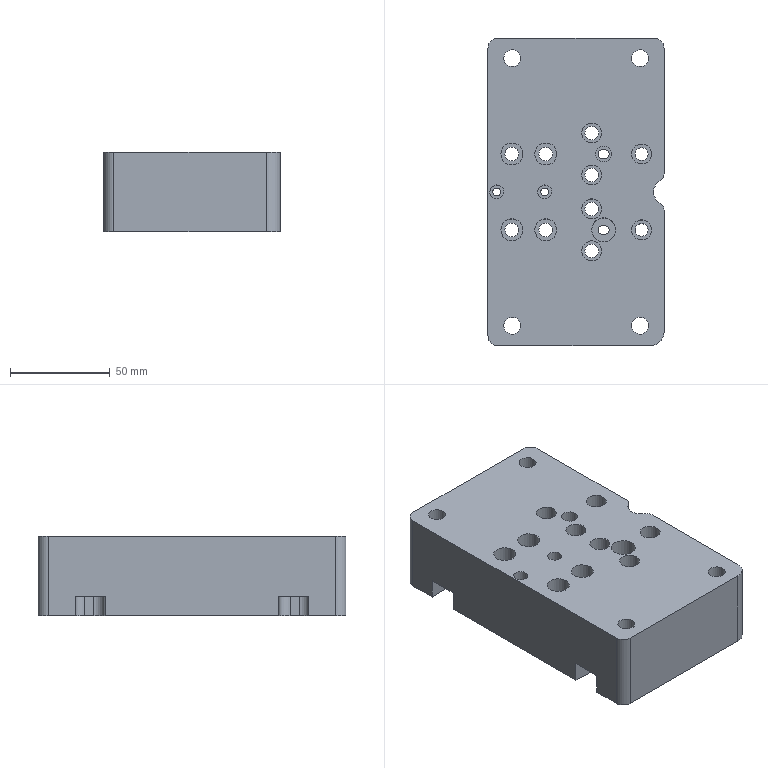Part | NX | features PS-40 2 | 1 solid | 102 faces | box 88.25 x 154 x 40 mm | volume 477533 mm3 | cylinder 57 | plane 45 | commonest cylinder face diameters 10 x21 6.9 x8 4.48 x4 8.5 x4 11 x4 14.5 x4